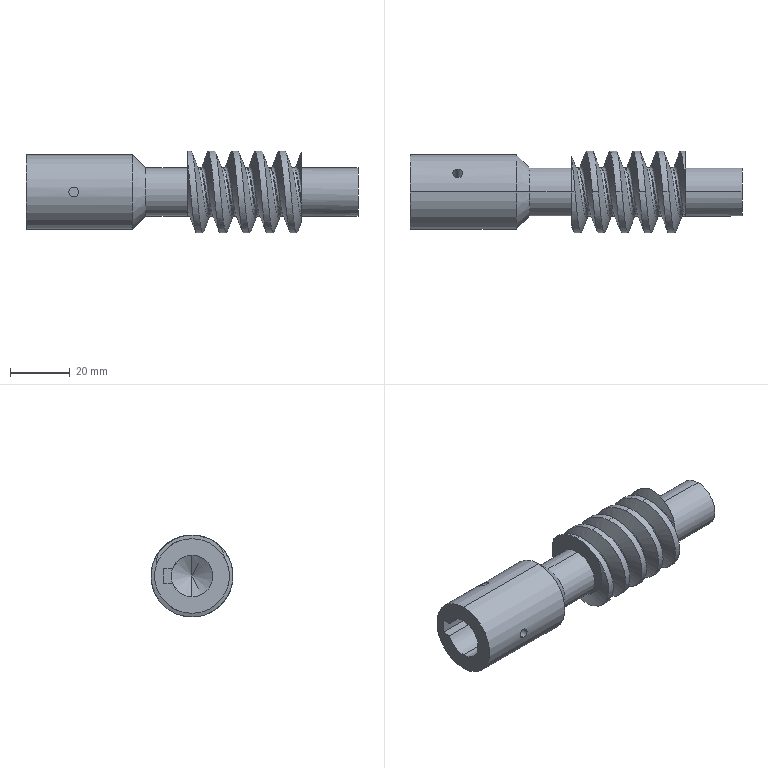Part | SolidWorks | features ICE 4, HoleWzd 2, Chamfer 1, CirPattern 1, Helix 1, RefAxis 1, Revolution 1, SweepCut 1 | 1 solid | 42 faces | box 111 x 27.4 x 27.4 mm | volume 34833 mm3 | cylinder 25 | plane 8 | spline 5 | cone 4 | commonest cylinder face diameters 27.4 x11 3.3 x6 16.15 x4 14 x2 25 x2